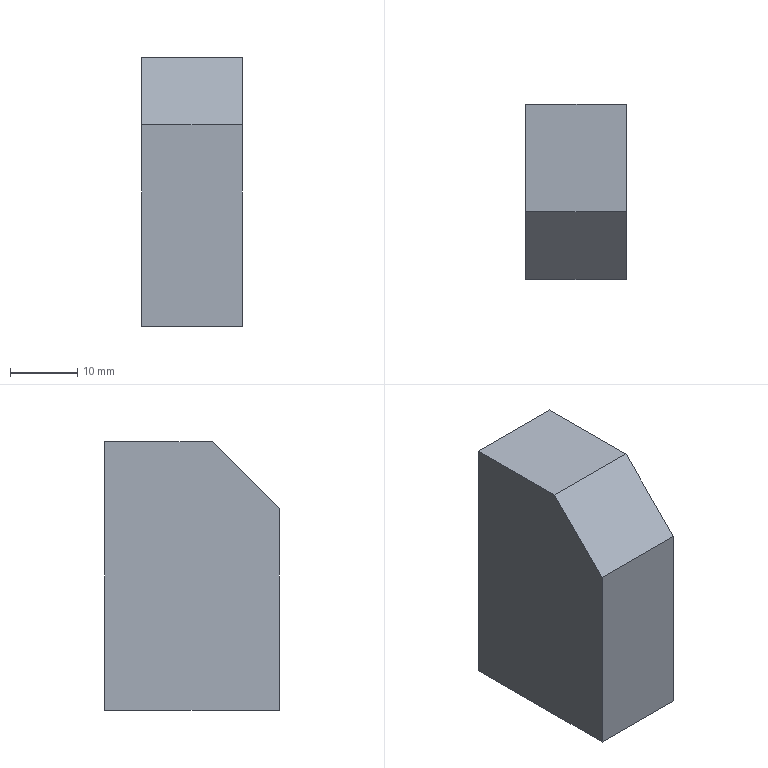Part | SolidWorks | features Chamfer 2, HoleWzd 2, Extrusion 1 | 1 solid | 23 faces | box 15 x 26 x 40 mm | volume 14020 mm3 | cylinder 10 | plane 7 | cone 6 | commonest cylinder face diameters 5 x10
STEP:
#1=CARTESIAN_POINT('',(0.,0.,16.502));
#2=VERTEX_POINT('',#1);
#3=CARTESIAN_POINT('',(-2.5,0.,15.));
#4=VERTEX_POINT('',#3);
#5=CARTESIAN_POINT('',(-2.5,0.,15.));
#6=DIRECTION('',(-0.8572,0.,-0.515));
#7=VECTOR('',#6,1000.);
#8=LINE('',#5,#7);
#9=EDGE_CURVE('',#2,#4,#8,.T.);
#10=ORIENTED_EDGE('',*,*,#9,.F.);
#11=CARTESIAN_POINT('',(2.5,0.,15.));
#12=VERTEX_POINT('',#11);
#13=CARTESIAN_POINT('',(2.5,0.,15.));
#14=DIRECTION('',(0.8572,0.,-0.515));
#15=VECTOR('',#14,1000.);
#16=LINE('',#13,#15);
#17=EDGE_CURVE('',#2,#12,#16,.T.);
#18=ORIENTED_EDGE('',*,*,#17,.T.);
#19=CARTESIAN_POINT('',(0.,0.,15.));
#20=DIRECTION('',(0.,0.,-1.));
#21=DIRECTION('',(-1.,0.,0.));
#22=AXIS2_PLACEMENT_3D('',#19,#20,#21);
#23=CIRCLE('',#22,2.5);
#24=EDGE_CURVE('',#12,#4,#23,.T.);
#25=ORIENTED_EDGE('',*,*,#24,.T.);
#26=EDGE_LOOP('',(#10,#18,#25));
#27=FACE_OUTER_BOUND('',#26,.T.);
#28=CARTESIAN_POINT('',(0.,0.,15.));
#29=DIRECTION('',(0.,0.,-1.));
#30=DIRECTION('',(-1.,0.,0.));
#31=AXIS2_PLACEMENT_3D('',#28,#29,#30);
#32=CONICAL_SURFACE('',#31,2.5,1.03);
#33=ADVANCED_FACE('',(#27),#32,.F.);
#34=ORIENTED_EDGE('',*,*,#24,.F.);
#35=CARTESIAN_POINT('',(2.5,0.,12.));
#36=VERTEX_POINT('',#35);
#37=CARTESIAN_POINT('',(2.5,0.,0.));
#38=DIRECTION('',(0.,0.,-1.));
#39=VECTOR('',#38,1000.);
#40=LINE('',#37,#39);
#41=EDGE_CURVE('',#12,#36,#40,.T.);
#42=ORIENTED_EDGE('',*,*,#41,.T.);
#43=CARTESIAN_POINT('',(1.5,-2.,14.));
#44=VERTEX_POINT('',#43);
#45=CARTESIAN_POINT('',(1.5,-2.,14.));
#46=CARTESIAN_POINT('',(2.141,-1.519,13.519));
#47=CARTESIAN_POINT('',(2.5,-0.8018,12.802));
#48=CARTESIAN_POINT('',(2.5,0.,12.));
#49=(BOUNDED_CURVE()B_SPLINE_CURVE(3,(#45,#46,#47,#48),.UNSPECIFIED.,.F.,.F.)B_SPLINE_CURVE_WITH_KNOTS((4,4),(3.785,4.712),.UNSPECIFIED.)CURVE()GEOMETRIC_REPRESENTATION_ITEM()RATIONAL_B_SPLINE_CURVE((1.,0.9296,0.9296,1.))REPRESENTATION_ITEM(''));
#50=EDGE_CURVE('',#44,#36,#49,.T.);
#51=ORIENTED_EDGE('',*,*,#50,.F.);
#52=CARTESIAN_POINT('',(0.,-2.5,13.668));
#53=VERTEX_POINT('',#52);
#54=CARTESIAN_POINT('',(0.,-2.5,13.668));
#55=CARTESIAN_POINT('',(0.1391,-2.5,13.668));
#56=CARTESIAN_POINT('',(0.279,-2.488,13.669));
#57=CARTESIAN_POINT('',(0.5511,-2.442,13.681));
#58=CARTESIAN_POINT('',(0.6845,-2.408,13.69));
#59=CARTESIAN_POINT('',(0.9452,-2.319,13.732));
#60=CARTESIAN_POINT('',(1.071,-2.263,13.764));
#61=CARTESIAN_POINT('',(1.3,-2.14,13.86));
#62=CARTESIAN_POINT('',(1.406,-2.071,13.924));
#63=CARTESIAN_POINT('',(1.5,-2.,14.));
#64=B_SPLINE_CURVE_WITH_KNOTS('',3,(#54,#55,#56,#57,#58,#59,#60,#61,#62,#63),.UNSPECIFIED.,.F.,.F.,(4,2,2,2,4),(0.001762,0.002177,0.002592,0.003008,0.003423),.UNSPECIFIED.);
#65=EDGE_CURVE('',#53,#44,#64,.T.);
#66=ORIENTED_EDGE('',*,*,#65,.F.);
#67=CARTESIAN_POINT('',(-1.5,-2.,14.));
#68=VERTEX_POINT('',#67);
#69=CARTESIAN_POINT('',(-1.5,-2.,14.));
#70=CARTESIAN_POINT('',(-1.406,-2.07,13.924));
#71=CARTESIAN_POINT('',(-1.303,-2.138,13.861));
#72=CARTESIAN_POINT('',(-1.071,-2.263,13.764));
#73=CARTESIAN_POINT('',(-0.9469,-2.318,13.732));
#74=CARTESIAN_POINT('',(-0.6869,-2.408,13.69));
#75=CARTESIAN_POINT('',(-0.5503,-2.443,13.68));
#76=CARTESIAN_POINT('',(-0.2772,-2.488,13.669));
#77=CARTESIAN_POINT('',(-0.1393,-2.5,13.668));
#78=CARTESIAN_POINT('',(0.,-2.5,13.668));
#79=B_SPLINE_CURVE_WITH_KNOTS('',3,(#69,#70,#71,#72,#73,#74,#75,#76,#77,#78),.UNSPECIFIED.,.F.,.F.,(4,2,2,2,4),(0.00009822,0.0005141,0.00093,0.001346,0.001762),.UNSPECIFIED.);
#80=EDGE_CURVE('',#68,#53,#79,.T.);
#81=ORIENTED_EDGE('',*,*,#80,.F.);
#82=CARTESIAN_POINT('',(-2.5,0.,12.));
#83=VERTEX_POINT('',#82);
#84=CARTESIAN_POINT('',(-2.5,0.,12.));
#85=CARTESIAN_POINT('',(-2.5,-0.8018,12.802));
#86=CARTESIAN_POINT('',(-2.141,-1.519,13.519));
#87=CARTESIAN_POINT('',(-1.5,-2.,14.));
#88=(BOUNDED_CURVE()B_SPLINE_CURVE(3,(#84,#85,#86,#87),.UNSPECIFIED.,.F.,.F.)B_SPLINE_CURVE_WITH_KNOTS((4,4),(1.571,2.498),.UNSPECIFIED.)CURVE()GEOMETRIC_REPRESENTATION_ITEM()RATIONAL_B_SPLINE_CURVE((1.,0.9296,0.9296,1.))REPRESENTATION_ITEM(''));
#89=EDGE_CURVE('',#83,#68,#88,.T.);
#90=ORIENTED_EDGE('',*,*,#89,.F.);
#91=CARTESIAN_POINT('',(-2.5,0.,0.));
#92=DIRECTION('',(0.,0.,-1.));
#93=VECTOR('',#92,1000.);
#94=LINE('',#91,#93);
#95=EDGE_CURVE('',#4,#83,#94,.T.);
#96=ORIENTED_EDGE('',*,*,#95,.F.);
#97=EDGE_LOOP('',(#34,#42,#51,#66,#81,#90,#96));
#98=FACE_OUTER_BOUND('',#97,.T.);
#99=CARTESIAN_POINT('',(0.,0.,0.));
#100=DIRECTION('',(0.,0.,-1.));
#101=DIRECTION('',(-1.,0.,0.));
#102=AXIS2_PLACEMENT_3D('',#99,#100,#101);
#103=CYLINDRICAL_SURFACE('',#102,2.5);
#104=ADVANCED_FACE('',(#98),#103,.F.);
#105=CARTESIAN_POINT('',(0.,-3.502,12.));
#106=VERTEX_POINT('',#105);
#107=CARTESIAN_POINT('',(0.,-2.,14.5));
#108=DIRECTION('',(0.,0.515,0.8572));
#109=VECTOR('',#108,1000.);
#110=LINE('',#107,#109);
#111=EDGE_CURVE('',#106,#53,#110,.T.);
#112=ORIENTED_EDGE('',*,*,#111,.F.);
#113=CARTESIAN_POINT('',(0.,-2.5,10.332));
#114=VERTEX_POINT('',#113);
#115=CARTESIAN_POINT('',(0.,-2.,9.5));
#116=DIRECTION('',(0.,0.515,-0.8572));
#117=VECTOR('',#116,1000.);
#118=LINE('',#115,#117);
#119=EDGE_CURVE('',#106,#114,#118,.T.);
#120=ORIENTED_EDGE('',*,*,#119,.T.);
#121=CARTESIAN_POINT('',(-1.5,-2.,10.));
#122=VERTEX_POINT('',#121);
#123=CARTESIAN_POINT('',(0.,-2.5,10.332));
#124=CARTESIAN_POINT('',(-0.1391,-2.5,10.332));
#125=CARTESIAN_POINT('',(-0.279,-2.488,10.331));
#126=CARTESIAN_POINT('',(-0.5511,-2.442,10.319));
#127=CARTESIAN_POINT('',(-0.6845,-2.408,10.31));
#128=CARTESIAN_POINT('',(-0.9452,-2.319,10.268));
#129=CARTESIAN_POINT('',(-1.071,-2.263,10.236));
#130=CARTESIAN_POINT('',(-1.3,-2.14,10.14));
#131=CARTESIAN_POINT('',(-1.406,-2.071,10.076));
#132=CARTESIAN_POINT('',(-1.5,-2.,10.));
#133=B_SPLINE_CURVE_WITH_KNOTS('',3,(#123,#124,#125,#126,#127,#128,#129,#130,#131,#132),.UNSPECIFIED.,.F.,.F.,(4,2,2,2,4),(0.001762,0.002177,0.002592,0.003008,0.003423),.UNSPECIFIED.);
#134=EDGE_CURVE('',#114,#122,#133,.T.);
#135=ORIENTED_EDGE('',*,*,#134,.T.);
#136=CARTESIAN_POINT('',(0.,-2.,12.));
#137=DIRECTION('',(0.,1.,0.));
#138=DIRECTION('',(0.,0.,1.));
#139=AXIS2_PLACEMENT_3D('',#136,#137,#138);
#140=CIRCLE('',#139,2.5);
#141=EDGE_CURVE('',#122,#68,#140,.T.);
#142=ORIENTED_EDGE('',*,*,#141,.T.);
#143=ORIENTED_EDGE('',*,*,#80,.T.);
#144=EDGE_LOOP('',(#112,#120,#135,#142,#143));
#145=FACE_OUTER_BOUND('',#144,.T.);
#146=CARTESIAN_POINT('',(0.,-2.,12.));
#147=DIRECTION('',(0.,1.,0.));
#148=DIRECTION('',(0.,0.,1.));
#149=AXIS2_PLACEMENT_3D('',#146,#147,#148);
#150=CONICAL_SURFACE('',#149,2.5,1.03);
#151=ADVANCED_FACE('',(#145),#150,.F.);
#152=CARTESIAN_POINT('',(1.5,-2.,10.));
#153=VERTEX_POINT('',#152);
#154=CARTESIAN_POINT('',(2.5,0.,12.));
#155=CARTESIAN_POINT('',(2.5,-0.8018,11.198));
#156=CARTESIAN_POINT('',(2.141,-1.519,10.481));
#157=CARTESIAN_POINT('',(1.5,-2.,10.));
#158=(BOUNDED_CURVE()B_SPLINE_CURVE(3,(#154,#155,#156,#157),.UNSPECIFIED.,.F.,.F.)B_SPLINE_CURVE_WITH_KNOTS((4,4),(1.571,2.498),.UNSPECIFIED.)CURVE()GEOMETRIC_REPRESENTATION_ITEM()RATIONAL_B_SPLINE_CURVE((1.,0.9296,0.9296,1.))REPRESENTATION_ITEM(''));
#159=EDGE_CURVE('',#36,#153,#158,.T.);
#160=ORIENTED_EDGE('',*,*,#159,.F.);
#161=CARTESIAN_POINT('',(2.5,0.,0.));
#162=VERTEX_POINT('',#161);
#163=CARTESIAN_POINT('',(2.5,0.,0.));
#164=DIRECTION('',(0.,0.,-1.));
#165=VECTOR('',#164,1000.);
#166=LINE('',#163,#165);
#167=EDGE_CURVE('',#36,#162,#166,.T.);
#168=ORIENTED_EDGE('',*,*,#167,.T.);
#169=CARTESIAN_POINT('',(-2.5,0.,0.));
#170=VERTEX_POINT('',#169);
#171=CARTESIAN_POINT('',(0.,0.,0.));
#172=DIRECTION('',(0.,0.,-1.));
#173=DIRECTION('',(-1.,0.,0.));
#174=AXIS2_PLACEMENT_3D('',#171,#172,#173);
#175=CIRCLE('',#174,2.5);
#176=EDGE_CURVE('',#162,#170,#175,.T.);
#177=ORIENTED_EDGE('',*,*,#176,.T.);
#178=CARTESIAN_POINT('',(-2.5,0.,0.));
#179=DIRECTION('',(0.,0.,-1.));
#180=VECTOR('',#179,1000.);
#181=LINE('',#178,#180);
#182=EDGE_CURVE('',#83,#170,#181,.T.);
#183=ORIENTED_EDGE('',*,*,#182,.F.);
#184=CARTESIAN_POINT('',(-1.5,-2.,10.));
#185=CARTESIAN_POINT('',(-2.141,-1.519,10.481));
#186=CARTESIAN_POINT('',(-2.5,-0.8018,11.198));
#187=CARTESIAN_POINT('',(-2.5,0.,12.));
#188=(BOUNDED_CURVE()B_SPLINE_CURVE(3,(#184,#185,#186,#187),.UNSPECIFIED.,.F.,.F.)B_SPLINE_CURVE_WITH_KNOTS((4,4),(3.785,4.712),.UNSPECIFIED.)CURVE()GEOMETRIC_REPRESENTATION_ITEM()RATIONAL_B_SPLINE_CURVE((1.,0.9296,0.9296,1.))REPRESENTATION_ITEM(''));
#189=EDGE_CURVE('',#122,#83,#188,.T.);
#190=ORIENTED_EDGE('',*,*,#189,.F.);
#191=ORIENTED_EDGE('',*,*,#134,.F.);
#192=CARTESIAN_POINT('',(1.5,-2.,10.));
#193=CARTESIAN_POINT('',(1.406,-2.07,10.076));
#194=CARTESIAN_POINT('',(1.303,-2.138,10.139));
#195=CARTESIAN_POINT('',(1.071,-2.263,10.236));
#196=CARTESIAN_POINT('',(0.9469,-2.318,10.268));
#197=CARTESIAN_POINT('',(0.6869,-2.408,10.31));
#198=CARTESIAN_POINT('',(0.5503,-2.443,10.32));
#199=CARTESIAN_POINT('',(0.2772,-2.488,10.331));
#200=CARTESIAN_POINT('',(0.1393,-2.5,10.332));
#201=CARTESIAN_POINT('',(0.,-2.5,10.332));
#202=B_SPLINE_CURVE_WITH_KNOTS('',3,(#192,#193,#194,#195,#196,#197,#198,#199,#200,#201),.UNSPECIFIED.,.F.,.F.,(4,2,2,2,4),(0.00009822,0.0005141,0.00093,0.001346,0.001762),.UNSPECIFIED.);
#203=EDGE_CURVE('',#153,#114,#202,.T.);
#204=ORIENTED_EDGE('',*,*,#203,.F.);
#205=EDGE_LOOP('',(#160,#168,#177,#183,#190,#191,#204));
#206=FACE_OUTER_BOUND('',#205,.T.);
#207=CARTESIAN_POINT('',(0.,0.,0.));
#208=DIRECTION('',(0.,0.,-1.));
#209=DIRECTION('',(-1.,0.,0.));
#210=AXIS2_PLACEMENT_3D('',#207,#208,#209);
#211=CYLINDRICAL_SURFACE('',#210,2.5);
#212=ADVANCED_FACE('',(#206),#211,.F.);
#213=CARTESIAN_POINT('',(0.,-2.,25.5));
#214=VERTEX_POINT('',#213);
#215=CARTESIAN_POINT('',(0.,-2.,30.5));
#216=VERTEX_POINT('',#215);
#217=CARTESIAN_POINT('',(0.,-2.,28.));
#218=DIRECTION('',(0.,1.,0.));
#219=DIRECTION('',(0.,0.,1.));
#220=AXIS2_PLACEMENT_3D('',#217,#218,#219);
#221=CIRCLE('',#220,2.5);
#222=EDGE_CURVE('',#214,#216,#221,.T.);
#223=ORIENTED_EDGE('',*,*,#222,.F.);
#224=CARTESIAN_POINT('',(0.,13.,25.5));
#225=VERTEX_POINT('',#224);
#226=CARTESIAN_POINT('',(0.,13.,25.5));
#227=DIRECTION('',(0.,1.,0.));
#228=VECTOR('',#227,1000.);
#229=LINE('',#226,#228);
#230=EDGE_CURVE('',#214,#225,#229,.T.);
#231=ORIENTED_EDGE('',*,*,#230,.T.);
#232=CARTESIAN_POINT('',(0.,13.,30.5));
#233=VERTEX_POINT('',#232);
#234=CARTESIAN_POINT('',(0.,13.,28.));
#235=DIRECTION('',(0.,1.,0.));
#236=DIRECTION('',(0.,0.,1.));
#237=AXIS2_PLACEMENT_3D('',#234,#235,#236);
#238=CIRCLE('',#237,2.5);
#239=EDGE_CURVE('',#225,#233,#238,.T.);
#240=ORIENTED_EDGE('',*,*,#239,.T.);
#241=CARTESIAN_POINT('',(0.,13.,30.5));
#242=DIRECTION('',(0.,1.,0.));
#243=VECTOR('',#242,1000.);
#244=LINE('',#241,#243);
#245=EDGE_CURVE('',#216,#233,#244,.T.);
#246=ORIENTED_EDGE('',*,*,#245,.F.);
#247=EDGE_LOOP('',(#223,#231,#240,#246));
#248=FACE_OUTER_BOUND('',#247,.T.);
#249=CARTESIAN_POINT('',(0.,13.,28.));
#250=DIRECTION('',(0.,1.,0.));
#251=DIRECTION('',(0.,0.,1.));
#252=AXIS2_PLACEMENT_3D('',#249,#250,#251);
#253=CYLINDRICAL_SURFACE('',#252,2.5);
#254=ADVANCED_FACE('',(#248),#253,.F.);
#255=CARTESIAN_POINT('',(0.,-3.502,28.));
#256=VERTEX_POINT('',#255);
#257=CARTESIAN_POINT('',(0.,-2.,30.5));
#258=DIRECTION('',(0.,0.515,0.8572));
#259=VECTOR('',#258,1000.);
#260=LINE('',#257,#259);
#261=EDGE_CURVE('',#256,#216,#260,.T.);
#262=ORIENTED_EDGE('',*,*,#261,.F.);
#263=CARTESIAN_POINT('',(0.,-2.,25.5));
#264=DIRECTION('',(0.,0.515,-0.8572));
#265=VECTOR('',#264,1000.);
#266=LINE('',#263,#265);
#267=EDGE_CURVE('',#256,#214,#266,.T.);
#268=ORIENTED_EDGE('',*,*,#267,.T.);
#269=ORIENTED_EDGE('',*,*,#222,.T.);
#270=EDGE_LOOP('',(#262,#268,#269));
#271=FACE_OUTER_BOUND('',#270,.T.);
#272=CARTESIAN_POINT('',(0.,-2.,28.));
#273=DIRECTION('',(0.,1.,0.));
#274=DIRECTION('',(0.,0.,1.));
#275=AXIS2_PLACEMENT_3D('',#272,#273,#274);
#276=CONICAL_SURFACE('',#275,2.5,1.03);
#277=ADVANCED_FACE('',(#271),#276,.F.);
#278=CARTESIAN_POINT('',(0.,2.5,9.5));
#279=VERTEX_POINT('',#278);
#280=CARTESIAN_POINT('',(-2.5,0.,12.));
#281=CARTESIAN_POINT('',(-2.5,1.464,10.536));
#282=CARTESIAN_POINT('',(-1.464,2.5,9.5));
#283=CARTESIAN_POINT('',(0.,2.5,9.5));
#284=(BOUNDED_CURVE()B_SPLINE_CURVE(3,(#280,#281,#282,#283),.UNSPECIFIED.,.F.,.F.)B_SPLINE_CURVE_WITH_KNOTS((4,4),(4.712,6.283),.UNSPECIFIED.)CURVE()GEOMETRIC_REPRESENTATION_ITEM()RATIONAL_B_SPLINE_CURVE((1.,0.8047,0.8047,1.))REPRESENTATION_ITEM(''));
#285=EDGE_CURVE('',#83,#279,#284,.T.);
#286=ORIENTED_EDGE('',*,*,#285,.T.);
#287=CARTESIAN_POINT('',(0.,13.,9.5));
#288=VERTEX_POINT('',#287);
#289=CARTESIAN_POINT('',(0.,13.,9.5));
#290=DIRECTION('',(0.,1.,0.));
#291=VECTOR('',#290,1000.);
#292=LINE('',#289,#291);
#293=EDGE_CURVE('',#279,#288,#292,.T.);
#294=ORIENTED_EDGE('',*,*,#293,.T.);
#295=CARTESIAN_POINT('',(0.,13.,14.5));
#296=VERTEX_POINT('',#295);
#297=CARTESIAN_POINT('',(0.,13.,12.));
#298=DIRECTION('',(0.,1.,0.));
#299=DIRECTION('',(0.,0.,1.));
#300=AXIS2_PLACEMENT_3D('',#297,#298,#299);
#301=CIRCLE('',#300,2.5);
#302=EDGE_CURVE('',#288,#296,#301,.T.);
#303=ORIENTED_EDGE('',*,*,#302,.T.);
#304=CARTESIAN_POINT('',(0.,2.5,14.5));
#305=VERTEX_POINT('',#304);
#306=CARTESIAN_POINT('',(0.,13.,14.5));
#307=DIRECTION('',(0.,1.,0.));
#308=VECTOR('',#307,1000.);
#309=LINE('',#306,#308);
#310=EDGE_CURVE('',#305,#296,#309,.T.);
#311=ORIENTED_EDGE('',*,*,#310,.F.);
#312=CARTESIAN_POINT('',(0.,2.5,14.5));
#313=CARTESIAN_POINT('',(-1.464,2.5,14.5));
#314=CARTESIAN_POINT('',(-2.5,1.464,13.464));
#315=CARTESIAN_POINT('',(-2.5,0.,12.));
#316=(BOUNDED_CURVE()B_SPLINE_CURVE(3,(#312,#313,#314,#315),.UNSPECIFIED.,.F.,.F.)B_SPLINE_CURVE_WITH_KNOTS((4,4),(0.,1.571),.UNSPECIFIED.)CURVE()GEOMETRIC_REPRESENTATION_ITEM()RATIONAL_B_SPLINE_CURVE((1.,0.8047,0.8047,1.))REPRESENTATION_ITEM(''));
#317=EDGE_CURVE('',#305,#83,#316,.T.);
#318=ORIENTED_EDGE('',*,*,#317,.T.);
#319=EDGE_LOOP('',(#286,#294,#303,#311,#318));
#320=FACE_OUTER_BOUND('',#319,.T.);
#321=CARTESIAN_POINT('',(0.,13.,12.));
#322=DIRECTION('',(0.,1.,0.));
#323=DIRECTION('',(0.,0.,1.));
#324=AXIS2_PLACEMENT_3D('',#321,#322,#323);
#325=CYLINDRICAL_SURFACE('',#324,2.5);
#326=ADVANCED_FACE('',(#320),#325,.F.);
#327=ORIENTED_EDGE('',*,*,#293,.F.);
#328=CARTESIAN_POINT('',(0.,2.5,9.5));
#329=CARTESIAN_POINT('',(1.464,2.5,9.5));
#330=CARTESIAN_POINT('',(2.5,1.464,10.536));
#331=CARTESIAN_POINT('',(2.5,0.,12.));
#332=(BOUNDED_CURVE()B_SPLINE_CURVE(3,(#328,#329,#330,#331),.UNSPECIFIED.,.F.,.F.)B_SPLINE_CURVE_WITH_KNOTS((4,4),(0.,1.571),.UNSPECIFIED.)CURVE()GEOMETRIC_REPRESENTATION_ITEM()RATIONAL_B_SPLINE_CURVE((1.,0.8047,0.8047,1.))REPRESENTATION_ITEM(''));
#333=EDGE_CURVE('',#279,#36,#332,.T.);
#334=ORIENTED_EDGE('',*,*,#333,.T.);
#335=CARTESIAN_POINT('',(2.5,0.,12.));
#336=CARTESIAN_POINT('',(2.5,1.464,13.464));
#337=CARTESIAN_POINT('',(1.464,2.5,14.5));
#338=CARTESIAN_POINT('',(0.,2.5,14.5));
#339=(BOUNDED_CURVE()B_SPLINE_CURVE(3,(#335,#336,#337,#338),.UNSPECIFIED.,.F.,.F.)B_SPLINE_CURVE_WITH_KNOTS((4,4),(4.712,6.283),.UNSPECIFIED.)CURVE()GEOMETRIC_REPRESENTATION_ITEM()RATIONAL_B_SPLINE_CURVE((1.,0.8047,0.8047,1.))REPRESENTATION_ITEM(''));
#340=EDGE_CURVE('',#36,#305,#339,.T.);
#341=ORIENTED_EDGE('',*,*,#340,.T.);
#342=ORIENTED_EDGE('',*,*,#310,.T.);
#343=CARTESIAN_POINT('',(0.,13.,12.));
#344=DIRECTION('',(0.,1.,0.));
#345=DIRECTION('',(0.,0.,1.));
#346=AXIS2_PLACEMENT_3D('',#343,#344,#345);
#347=CIRCLE('',#346,2.5);
#348=EDGE_CURVE('',#296,#288,#347,.T.);
#349=ORIENTED_EDGE('',*,*,#348,.T.);
#350=EDGE_LOOP('',(#327,#334,#341,#342,#349));
#351=FACE_OUTER_BOUND('',#350,.T.);
#352=CARTESIAN_POINT('',(0.,13.,12.));
#353=DIRECTION('',(0.,1.,0.));
#354=DIRECTION('',(0.,0.,1.));
#355=AXIS2_PLACEMENT_3D('',#352,#353,#354);
#356=CYLINDRICAL_SURFACE('',#355,2.5);
#357=ADVANCED_FACE('',(#351),#356,.F.);
#358=CARTESIAN_POINT('',(7.5,-3.,40.));
#359=VERTEX_POINT('',#358);
#360=CARTESIAN_POINT('',(7.5,13.,40.));
#361=VERTEX_POINT('',#360);
#362=CARTESIAN_POINT('',(7.5,13.,40.));
#363=DIRECTION('',(0.,1.,0.));
#364=VECTOR('',#363,1000.);
#365=LINE('',#362,#364);
#366=EDGE_CURVE('',#359,#361,#365,.T.);
#367=ORIENTED_EDGE('',*,*,#366,.F.);
#368=CARTESIAN_POINT('',(7.5,-13.,30.));
#369=VERTEX_POINT('',#368);
#370=CARTESIAN_POINT('',(7.5,-3.,40.));
#371=DIRECTION('',(0.,-0.7071,-0.7071));
#372=VECTOR('',#371,1000.);
#373=LINE('',#370,#372);
#374=EDGE_CURVE('',#359,#369,#373,.T.);
#375=ORIENTED_EDGE('',*,*,#374,.T.);
#376=CARTESIAN_POINT('',(7.5,-13.,0.));
#377=VERTEX_POINT('',#376);
#378=CARTESIAN_POINT('',(7.5,-13.,40.));
#379=DIRECTION('',(0.,0.,-1.));
#380=VECTOR('',#379,1000.);
#381=LINE('',#378,#380);
#382=EDGE_CURVE('',#369,#377,#381,.T.);
#383=ORIENTED_EDGE('',*,*,#382,.T.);
#384=CARTESIAN_POINT('',(7.5,13.,0.));
#385=VERTEX_POINT('',#384);
#386=CARTESIAN_POINT('',(7.5,13.,0.));
#387=DIRECTION('',(0.,1.,0.));
#388=VECTOR('',#387,1000.);
#389=LINE('',#386,#388);
#390=EDGE_CURVE('',#377,#385,#389,.T.);
#391=ORIENTED_EDGE('',*,*,#390,.T.);
#392=CARTESIAN_POINT('',(7.5,13.,40.));
#393=DIRECTION('',(0.,0.,-1.));
#394=VECTOR('',#393,1000.);
#395=LINE('',#392,#394);
#396=EDGE_CURVE('',#361,#385,#395,.T.);
#397=ORIENTED_EDGE('',*,*,#396,.F.);
#398=EDGE_LOOP('',(#367,#375,#383,#391,#397));
#399=FACE_OUTER_BOUND('',#398,.T.);
#400=CARTESIAN_POINT('',(7.5,13.,40.));
#401=DIRECTION('',(-1.,0.,0.));
#402=DIRECTION('',(0.,-1.,0.));
#403=AXIS2_PLACEMENT_3D('',#400,#401,#402);
#404=PLANE('',#403);
#405=ADVANCED_FACE('',(#399),#404,.F.);
#406=ORIENTED_EDGE('',*,*,#348,.F.);
#407=ORIENTED_EDGE('',*,*,#302,.F.);
#408=EDGE_LOOP('',(#406,#407));
#409=FACE_BOUND('',#408,.T.);
#410=CARTESIAN_POINT('',(0.,13.,28.));
#411=DIRECTION('',(0.,1.,0.));
#412=DIRECTION('',(0.,0.,1.));
#413=AXIS2_PLACEMENT_3D('',#410,#411,#412);
#414=CIRCLE('',#413,2.5);
#415=EDGE_CURVE('',#233,#225,#414,.T.);
#416=ORIENTED_EDGE('',*,*,#415,.F.);
#417=ORIENTED_EDGE('',*,*,#239,.F.);
#418=EDGE_LOOP('',(#416,#417));
#419=FACE_BOUND('',#418,.T.);
#420=CARTESIAN_POINT('',(-7.5,13.,0.));
#421=VERTEX_POINT('',#420);
#422=CARTESIAN_POINT('',(-7.5,13.,0.));
#423=DIRECTION('',(-1.,0.,0.));
#424=VECTOR('',#423,1000.);
#425=LINE('',#422,#424);
#426=EDGE_CURVE('',#385,#421,#425,.T.);
#427=ORIENTED_EDGE('',*,*,#426,.T.);
#428=CARTESIAN_POINT('',(-7.5,13.,40.));
#429=VERTEX_POINT('',#428);
#430=CARTESIAN_POINT('',(-7.5,13.,40.));
#431=DIRECTION('',(0.,0.,-1.));
#432=VECTOR('',#431,1000.);
#433=LINE('',#430,#432);
#434=EDGE_CURVE('',#429,#421,#433,.T.);
#435=ORIENTED_EDGE('',*,*,#434,.F.);
#436=CARTESIAN_POINT('',(-7.5,13.,40.));
#437=DIRECTION('',(-1.,0.,0.));
#438=VECTOR('',#437,1000.);
#439=LINE('',#436,#438);
#440=EDGE_CURVE('',#361,#429,#439,.T.);
#441=ORIENTED_EDGE('',*,*,#440,.F.);
#442=ORIENTED_EDGE('',*,*,#396,.T.);
#443=EDGE_LOOP('',(#427,#435,#441,#442));
#444=FACE_OUTER_BOUND('',#443,.T.);
#445=CARTESIAN_POINT('',(-7.5,13.,40.));
#446=DIRECTION('',(0.,-1.,0.));
#447=DIRECTION('',(0.,0.,-1.));
#448=AXIS2_PLACEMENT_3D('',#445,#446,#447);
#449=PLANE('',#448);
#450=ADVANCED_FACE('',(#409,#419,#444),#449,.F.);
#451=CARTESIAN_POINT('',(-7.5,-13.,30.));
#452=VERTEX_POINT('',#451);
#453=CARTESIAN_POINT('',(-7.5,-13.,0.));
#454=VERTEX_POINT('',#453);
#455=CARTESIAN_POINT('',(-7.5,-13.,40.));
#456=DIRECTION('',(0.,0.,-1.));
#457=VECTOR('',#456,1000.);
#458=LINE('',#455,#457);
#459=EDGE_CURVE('',#452,#454,#458,.T.);
#460=ORIENTED_EDGE('',*,*,#459,.F.);
#461=CARTESIAN_POINT('',(-7.5,-3.,40.));
#462=VERTEX_POINT('',#461);
#463=CARTESIAN_POINT('',(-7.5,-3.,40.));
#464=DIRECTION('',(0.,0.7071,0.7071));
#465=VECTOR('',#464,1000.);
#466=LINE('',#463,#465);
#467=EDGE_CURVE('',#452,#462,#466,.T.);
#468=ORIENTED_EDGE('',*,*,#467,.T.);
#469=CARTESIAN_POINT('',(-7.5,13.,40.));
#470=DIRECTION('',(0.,-1.,0.));
#471=VECTOR('',#470,1000.);
#472=LINE('',#469,#471);
#473=EDGE_CURVE('',#429,#462,#472,.T.);
#474=ORIENTED_EDGE('',*,*,#473,.F.);
#475=ORIENTED_EDGE('',*,*,#434,.T.);
#476=CARTESIAN_POINT('',(-7.5,13.,0.));
#477=DIRECTION('',(0.,-1.,0.));
#478=VECTOR('',#477,1000.);
#479=LINE('',#476,#478);
#480=EDGE_CURVE('',#421,#454,#479,.T.);
#481=ORIENTED_EDGE('',*,*,#480,.T.);
#482=EDGE_LOOP('',(#460,#468,#474,#475,#481));
#483=FACE_OUTER_BOUND('',#482,.T.);
#484=CARTESIAN_POINT('',(-7.5,13.,40.));
#485=DIRECTION('',(1.,0.,0.));
#486=DIRECTION('',(0.,1.,0.));
#487=AXIS2_PLACEMENT_3D('',#484,#485,#486);
#488=PLANE('',#487);
#489=ADVANCED_FACE('',(#483),#488,.F.);
#490=ORIENTED_EDGE('',*,*,#382,.F.);
#491=CARTESIAN_POINT('',(-7.5,-13.,30.));
#492=DIRECTION('',(-1.,0.,0.));
#493=VECTOR('',#492,1000.);
#494=LINE('',#491,#493);
#495=EDGE_CURVE('',#369,#452,#494,.T.);
#496=ORIENTED_EDGE('',*,*,#495,.T.);
#497=ORIENTED_EDGE('',*,*,#459,.T.);
#498=CARTESIAN_POINT('',(-7.5,-13.,0.));
#499=DIRECTION('',(1.,0.,0.));
#500=VECTOR('',#499,1000.);
#501=LINE('',#498,#500);
#502=EDGE_CURVE('',#454,#377,#501,.T.);
#503=ORIENTED_EDGE('',*,*,#502,.T.);
#504=EDGE_LOOP('',(#490,#496,#497,#503));
#505=FACE_OUTER_BOUND('',#504,.T.);
#506=CARTESIAN_POINT('',(-7.5,-13.,40.));
#507=DIRECTION('',(0.,1.,0.));
#508=DIRECTION('',(0.,0.,1.));
#509=AXIS2_PLACEMENT_3D('',#506,#507,#508);
#510=PLANE('',#509);
#511=ADVANCED_FACE('',(#505),#510,.F.);
#512=ORIENTED_EDGE('',*,*,#473,.T.);
#513=CARTESIAN_POINT('',(7.5,-3.,40.));
#514=DIRECTION('',(1.,0.,0.));
#515=VECTOR('',#514,1000.);
#516=LINE('',#513,#515);
#517=EDGE_CURVE('',#462,#359,#516,.T.);
#518=ORIENTED_EDGE('',*,*,#517,.T.);
#519=ORIENTED_EDGE('',*,*,#366,.T.);
#520=ORIENTED_EDGE('',*,*,#440,.T.);
#521=EDGE_LOOP('',(#512,#518,#519,#520));
#522=FACE_OUTER_BOUND('',#521,.T.);
#523=CARTESIAN_POINT('',(0.,0.,40.));
#524=DIRECTION('',(0.,0.,1.));
#525=DIRECTION('',(1.,0.,0.));
#526=AXIS2_PLACEMENT_3D('',#523,#524,#525);
#527=PLANE('',#526);
#528=ADVANCED_FACE('',(#522),#527,.T.);
#529=CARTESIAN_POINT('',(0.,0.,0.));
#530=DIRECTION('',(0.,0.,-1.));
#531=DIRECTION('',(-1.,0.,0.));
#532=AXIS2_PLACEMENT_3D('',#529,#530,#531);
#533=CIRCLE('',#532,2.5);
#534=EDGE_CURVE('',#170,#162,#533,.T.);
#535=ORIENTED_EDGE('',*,*,#534,.F.);
#536=ORIENTED_EDGE('',*,*,#176,.F.);
#537=EDGE_LOOP('',(#535,#536));
#538=FACE_BOUND('',#537,.T.);
#539=ORIENTED_EDGE('',*,*,#390,.F.);
#540=ORIENTED_EDGE('',*,*,#502,.F.);
#541=ORIENTED_EDGE('',*,*,#480,.F.);
#542=ORIENTED_EDGE('',*,*,#426,.F.);
#543=EDGE_LOOP('',(#539,#540,#541,#542));
#544=FACE_OUTER_BOUND('',#543,.T.);
#545=CARTESIAN_POINT('',(0.,0.,0.));
#546=DIRECTION('',(0.,0.,1.));
#547=DIRECTION('',(1.,0.,0.));
#548=AXIS2_PLACEMENT_3D('',#545,#546,#547);
#549=PLANE('',#548);
#550=ADVANCED_FACE('',(#538,#544),#549,.F.);
#551=ORIENTED_EDGE('',*,*,#267,.F.);
#552=ORIENTED_EDGE('',*,*,#261,.T.);
#553=CARTESIAN_POINT('',(0.,-2.,28.));
#554=DIRECTION('',(0.,1.,0.));
#555=DIRECTION('',(0.,0.,1.));
#556=AXIS2_PLACEMENT_3D('',#553,#554,#555);
#557=CIRCLE('',#556,2.5);
#558=EDGE_CURVE('',#216,#214,#557,.T.);
#559=ORIENTED_EDGE('',*,*,#558,.T.);
#560=EDGE_LOOP('',(#551,#552,#559));
#561=FACE_OUTER_BOUND('',#560,.T.);
#562=CARTESIAN_POINT('',(0.,-2.,28.));
#563=DIRECTION('',(0.,1.,0.));
#564=DIRECTION('',(0.,0.,1.));
#565=AXIS2_PLACEMENT_3D('',#562,#563,#564);
#566=CONICAL_SURFACE('',#565,2.5,1.03);
#567=ADVANCED_FACE('',(#561),#566,.F.);
#568=ORIENTED_EDGE('',*,*,#230,.F.);
#569=ORIENTED_EDGE('',*,*,#558,.F.);
#570=ORIENTED_EDGE('',*,*,#245,.T.);
#571=ORIENTED_EDGE('',*,*,#415,.T.);
#572=EDGE_LOOP('',(#568,#569,#570,#571));
#573=FACE_OUTER_BOUND('',#572,.T.);
#574=CARTESIAN_POINT('',(0.,13.,28.));
#575=DIRECTION('',(0.,1.,0.));
#576=DIRECTION('',(0.,0.,1.));
#577=AXIS2_PLACEMENT_3D('',#574,#575,#576);
#578=CYLINDRICAL_SURFACE('',#577,2.5);
#579=ADVANCED_FACE('',(#573),#578,.F.);
#580=ORIENTED_EDGE('',*,*,#167,.F.);
#581=ORIENTED_EDGE('',*,*,#333,.F.);
#582=ORIENTED_EDGE('',*,*,#285,.F.);
#583=ORIENTED_EDGE('',*,*,#182,.T.);
#584=ORIENTED_EDGE('',*,*,#534,.T.);
#585=EDGE_LOOP('',(#580,#581,#582,#583,#584));
#586=FACE_OUTER_BOUND('',#585,.T.);
#587=CARTESIAN_POINT('',(0.,0.,0.));
#588=DIRECTION('',(0.,0.,-1.));
#589=DIRECTION('',(-1.,0.,0.));
#590=AXIS2_PLACEMENT_3D('',#587,#588,#589);
#591=CYLINDRICAL_SURFACE('',#590,2.5);
#592=ADVANCED_FACE('',(#586),#591,.F.);
#593=ORIENTED_EDGE('',*,*,#50,.T.);
#594=ORIENTED_EDGE('',*,*,#159,.T.);
#595=CARTESIAN_POINT('',(0.,-2.,12.));
#596=DIRECTION('',(0.,1.,0.));
#597=DIRECTION('',(0.,0.,1.));
#598=AXIS2_PLACEMENT_3D('',#595,#596,#597);
#599=CIRCLE('',#598,2.5);
#600=EDGE_CURVE('',#44,#153,#599,.T.);
#601=ORIENTED_EDGE('',*,*,#600,.F.);
#602=EDGE_LOOP('',(#593,#594,#601));
#603=FACE_OUTER_BOUND('',#602,.T.);
#604=CARTESIAN_POINT('',(0.,13.,12.));
#605=DIRECTION('',(0.,1.,0.));
#606=DIRECTION('',(0.,0.,1.));
#607=AXIS2_PLACEMENT_3D('',#604,#605,#606);
#608=CYLINDRICAL_SURFACE('',#607,2.5);
#609=ADVANCED_FACE('',(#603),#608,.F.);
#610=ORIENTED_EDGE('',*,*,#141,.F.);
#611=ORIENTED_EDGE('',*,*,#189,.T.);
#612=ORIENTED_EDGE('',*,*,#89,.T.);
#613=EDGE_LOOP('',(#610,#611,#612));
#614=FACE_OUTER_BOUND('',#613,.T.);
#615=CARTESIAN_POINT('',(0.,13.,12.));
#616=DIRECTION('',(0.,1.,0.));
#617=DIRECTION('',(0.,0.,1.));
#618=AXIS2_PLACEMENT_3D('',#615,#616,#617);
#619=CYLINDRICAL_SURFACE('',#618,2.5);
#620=ADVANCED_FACE('',(#614),#619,.F.);
#621=ORIENTED_EDGE('',*,*,#119,.F.);
#622=ORIENTED_EDGE('',*,*,#111,.T.);
#623=ORIENTED_EDGE('',*,*,#65,.T.);
#624=ORIENTED_EDGE('',*,*,#600,.T.);
#625=ORIENTED_EDGE('',*,*,#203,.T.);
#626=EDGE_LOOP('',(#621,#622,#623,#624,#625));
#627=FACE_OUTER_BOUND('',#626,.T.);
#628=CARTESIAN_POINT('',(0.,-2.,12.));
#629=DIRECTION('',(0.,1.,0.));
#630=DIRECTION('',(0.,0.,1.));
#631=AXIS2_PLACEMENT_3D('',#628,#629,#630);
#632=CONICAL_SURFACE('',#631,2.5,1.03);
#633=ADVANCED_FACE('',(#627),#632,.F.);
#634=ORIENTED_EDGE('',*,*,#41,.F.);
#635=CARTESIAN_POINT('',(0.,0.,15.));
#636=DIRECTION('',(0.,0.,-1.));
#637=DIRECTION('',(-1.,0.,0.));
#638=AXIS2_PLACEMENT_3D('',#635,#636,#637);
#639=CIRCLE('',#638,2.5);
#640=EDGE_CURVE('',#4,#12,#639,.T.);
#641=ORIENTED_EDGE('',*,*,#640,.F.);
#642=ORIENTED_EDGE('',*,*,#95,.T.);
#643=ORIENTED_EDGE('',*,*,#317,.F.);
#644=ORIENTED_EDGE('',*,*,#340,.F.);
#645=EDGE_LOOP('',(#634,#641,#642,#643,#644));
#646=FACE_OUTER_BOUND('',#645,.T.);
#647=CARTESIAN_POINT('',(0.,0.,0.));
#648=DIRECTION('',(0.,0.,-1.));
#649=DIRECTION('',(-1.,0.,0.));
#650=AXIS2_PLACEMENT_3D('',#647,#648,#649);
#651=CYLINDRICAL_SURFACE('',#650,2.5);
#652=ADVANCED_FACE('',(#646),#651,.F.);
#653=ORIENTED_EDGE('',*,*,#17,.F.);
#654=ORIENTED_EDGE('',*,*,#9,.T.);
#655=ORIENTED_EDGE('',*,*,#640,.T.);
#656=EDGE_LOOP('',(#653,#654,#655));
#657=FACE_OUTER_BOUND('',#656,.T.);
#658=CARTESIAN_POINT('',(0.,0.,15.));
#659=DIRECTION('',(0.,0.,-1.));
#660=DIRECTION('',(-1.,0.,0.));
#661=AXIS2_PLACEMENT_3D('',#658,#659,#660);
#662=CONICAL_SURFACE('',#661,2.5,1.03);
#663=ADVANCED_FACE('',(#657),#662,.F.);
#664=ORIENTED_EDGE('',*,*,#467,.F.);
#665=ORIENTED_EDGE('',*,*,#495,.F.);
#666=ORIENTED_EDGE('',*,*,#374,.F.);
#667=ORIENTED_EDGE('',*,*,#517,.F.);
#668=EDGE_LOOP('',(#664,#665,#666,#667));
#669=FACE_OUTER_BOUND('',#668,.T.);
#670=CARTESIAN_POINT('',(0.,-3.,40.));
#671=DIRECTION('',(0.,-0.7071,0.7071));
#672=DIRECTION('',(-1.,0.,0.));
#673=AXIS2_PLACEMENT_3D('',#670,#671,#672);
#674=PLANE('',#673);
#675=ADVANCED_FACE('',(#669),#674,.T.);
#676=CLOSED_SHELL('',(#33,#104,#151,#212,#254,#277,#326,#357,#405,#450,#489,#511,#528,#550,#567,#579,#592,#609,#620,#633,#652,#663,#675));
#677=MANIFOLD_SOLID_BREP('',#676);
#678=CARTESIAN_POINT('',(0.,0.,0.));
#679=DIRECTION('',(0.,0.,1.));
#680=DIRECTION('',(1.,0.,0.));
#681=AXIS2_PLACEMENT_3D('',#678,#679,#680);
#682=(LENGTH_UNIT()NAMED_UNIT(*)SI_UNIT(.MILLI.,.METRE.));
#683=UNCERTAINTY_MEASURE_WITH_UNIT(LENGTH_MEASURE(0.00001),#682,'','');
#684=(NAMED_UNIT(*)PLANE_ANGLE_UNIT()SI_UNIT($,.RADIAN.));
#685=(NAMED_UNIT(*)SI_UNIT($,.STERADIAN.)SOLID_ANGLE_UNIT());
#686=(GEOMETRIC_REPRESENTATION_CONTEXT(3)GLOBAL_UNCERTAINTY_ASSIGNED_CONTEXT((#683))GLOBAL_UNIT_ASSIGNED_CONTEXT((#682,#684,#685))REPRESENTATION_CONTEXT('',''));
#687=ADVANCED_BREP_SHAPE_REPRESENTATION('',(#677,#681),#686);